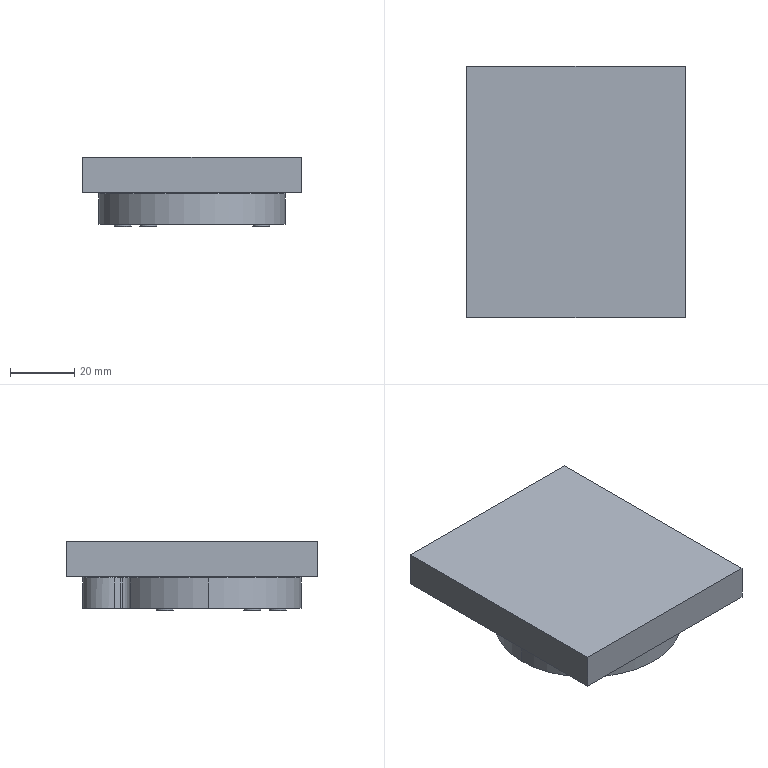NC program | NX | posted with a generic post | part box 68 x 78.27 x 21.8 mm
Lines 1 to 1194 of 3502:
N10 G17 G21 G94 G90
(FLOOR_WALL , TOOL : D80)
N12 T19 M6
N14 G54
N16 G17 G0 G90 X-74. Y0. S5000 M3
N18 G43 Z30. H19
N20 Z3.
N22 G94 G1 Z0. F1200.
N24 X-71.
N26 X71.
N28 X74.
N30 Z3.
N32 G0 Z30.
N34 M5
(CAVITY_MILL , TOOL : D10)
N36 T15 M6
N38 G54
N40 G17 G0 G90 X-37.995 Y9.548 S9500 M3
N42 G43 Z30. H15
N44 Z0.525
N46 G94 G1 Z-0.975 F1000.
N48 X-31.995 Y13.012
N50 G3 X-31.495 Y13.879 R1.
N52 G1 Y36.139 F3500.
N54 G2 X-31.003 Y36.632 R0.492
N56 G1 X31.003
N58 G2 X31.495 Y36.139 R0.492
N60 G1 Y-36.139
N62 G2 X31.003 Y-36.632 R0.492
N64 G1 X-31.003
N66 G2 X-31.495 Y-36.139 R0.492
N68 G1 Y13.879
N70 X-25.495
N72 Y30.632
N74 X25.495
N76 Y-30.632
N78 X-25.495
N80 Y13.879
N82 X-19.495
N84 Y24.632
N86 X19.495
N88 Y-24.632
N90 X9.149
N92 Y-18.632
N94 G3 X13.495 Y-14.286 R16.305
N96 G1 Y-18.632
N98 X9.149
N100 Y-24.632
N102 X-19.495
N104 Y-14.286
N106 X-13.495
N108 G3 X-9.149 Y-18.632 R16.305
N110 G1 X-13.495
N112 Y-14.286
N114 X-19.495
N116 Y13.879
N118 X-13.495
N120 Y18.632
N122 X13.495
N124 Y4.016
N126 G3 X6.155 Y9.964 R16.306
N128 G1 X7.853 Y14.132
N130 X8.995
N132 Y13.626
N134 G3 X7.853 Y14.132 R20.805
N136 G1 X6.155 Y9.964
N138 G3 X-13.495 Y4.016 R16.305
N140 G1 X-12.502 Y3.343
N142 G2 X8.478 Y7.367 R15.105
N144 X-12.502 Y3.343 R-15.105
N146 G1 X-13.495 Y4.016
N148 Y13.879
N150 X-8.995
N152 Y14.132
N154 X-7.853
N156 G3 X-8.995 Y13.626 R20.805
N158 G1 Y13.879
N160 G3 X-9.495 Y14.745 R1.
N162 G1 Z0.525
N164 G0 Z30.
N166 X-37.996 Y9.548
N168 Z-0.45
N170 G1 Z-1.95 F1000.
N172 X-31.996 Y13.013
N174 G3 X-31.496 Y13.879 R1.
N176 G1 Y36.139 F3500.
N178 G2 X-31.003 Y36.632 R0.493
N180 G1 X31.003
N182 G2 X31.496 Y36.139 R0.493
N184 G1 Y-36.139
N186 G2 X31.003 Y-36.632 R0.493
N188 G1 X-31.003
N190 G2 X-31.496 Y-36.139 R0.493
N192 G1 Y13.879
N194 X-25.496
N196 Y30.632
N198 X25.496
N200 Y-30.632
N202 X-25.496
N204 Y13.879
N206 X-19.496
N208 Y24.632
N210 X19.496
N212 Y-24.632
N214 X9.149
N216 Y-18.632
N218 G3 X13.496 Y-14.286 R16.305
N220 G1 Y-18.632
N222 X9.149
N224 Y-24.632
N226 X-19.496
N228 Y-14.286
N230 X-13.496
N232 G3 X-9.149 Y-18.632 R16.305
N234 G1 X-13.496
N236 Y-14.286
N238 X-19.496
N240 Y13.879
N242 X-13.496
N244 Y18.632
N246 X13.496
N248 Y4.016
N250 G3 X6.154 Y9.965 R16.306
N252 G1 X7.853 Y14.132
N254 X8.996
N256 Y13.625
N258 G3 X7.853 Y14.132 R20.805
N260 G1 X6.154 Y9.965
N262 G3 X-13.496 Y4.016 R16.305
N264 G1 X-12.502 Y3.342
N266 G2 X8.477 Y7.368 R15.105
N268 X-12.502 Y3.342 R-15.105
N270 G1 X-13.496 Y4.016
N272 Y13.879
N274 X-8.996
N276 Y14.132
N278 X-7.853
N280 G3 X-8.996 Y13.625 R20.805
N282 G1 Y13.879
N284 G3 X-9.496 Y14.745 R1.
N286 G1 Z-0.45
N288 G0 Z2.025
N290 X-37.996 Y9.548
N292 Z-1.425
N294 G1 Z-2.925 F1000.
N296 X-31.996 Y13.013
N298 G3 X-31.496 Y13.879 R1.
N300 G1 Y36.139 F3500.
N302 G2 X-31.003 Y36.632 R0.493
N304 G1 X31.003
N306 G2 X31.496 Y36.139 R0.493
N308 G1 Y-36.139
N310 G2 X31.003 Y-36.632 R0.493
N312 G1 X-31.003
N314 G2 X-31.496 Y-36.139 R0.493
N316 G1 Y13.879
N318 X-25.496
N320 Y30.632
N322 X25.496
N324 Y-30.632
N326 X-25.496
N328 Y13.879
N330 X-19.496
N332 Y24.632
N334 X19.496
N336 Y-24.632
N338 X9.149
N340 Y-18.632
N342 G3 X13.496 Y-14.285 R16.305
N344 G1 Y-18.632
N346 X9.149
N348 Y-24.632
N350 X-19.496
N352 Y-14.285
N354 X-13.496
N356 G3 X-9.149 Y-18.632 R16.305
N358 G1 X-13.496
N360 Y-14.285
N362 X-19.496
N364 Y13.879
N366 X-13.496
N368 Y18.632
N370 X13.496
N372 Y4.016
N374 G3 X6.154 Y9.965 R16.305
N376 G1 X7.852 Y14.132
N378 X8.996
N380 Y13.625
N382 G3 X7.852 Y14.132 R20.805
N384 G1 X6.154 Y9.965
N386 G3 X-13.496 Y4.016 R16.305
N388 G1 X-12.503 Y3.342
N390 G2 X8.477 Y7.368 R15.105
N392 X-12.503 Y3.342 R-15.105
N394 G1 X-13.496 Y4.016
N396 Y13.879
N398 X-8.996
N400 Y14.132
N402 X-7.852
N404 G3 X-8.996 Y13.625 R20.805
N406 G1 Y13.879
N408 G3 X-9.496 Y14.745 R1.
N410 G1 Z-1.425
N412 G0 Z1.05
N414 X-37.996 Y9.549
N416 Z-2.4
N418 G1 Z-3.9 F1000.
N420 X-31.996 Y13.013
N422 G3 X-31.496 Y13.879 R1.
N424 G1 Y36.139 F3500.
N426 G2 X-31.003 Y36.632 R0.493
N428 G1 X31.003
N430 G2 X31.496 Y36.139 R0.493
N432 G1 Y-36.139
N434 G2 X31.003 Y-36.632 R0.493
N436 G1 X-31.003
N438 G2 X-31.496 Y-36.139 R0.493
N440 G1 Y13.879
N442 X-25.496
N444 Y30.632
N446 X25.496
N448 Y-30.632
N450 X-25.496
N452 Y13.879
N454 X-19.496
N456 Y24.632
N458 X19.496
N460 Y-24.632
N462 X9.148
N464 Y-18.632
N466 G3 X13.496 Y-14.285 R16.305
N468 G1 Y-18.632
N470 X9.148
N472 Y-24.632
N474 X-19.496
N476 Y-14.285
N478 X-13.496
N480 G3 X-9.148 Y-18.632 R16.305
N482 G1 X-13.496
N484 Y-14.285
N486 X-19.496
N488 Y13.879
N490 X-13.496
N492 Y18.632
N494 X13.496
N496 Y4.015
N498 G3 X6.154 Y9.965 R16.305
N500 G1 X7.852 Y14.132
N502 X8.996
N504 Y13.625
N506 G3 X7.852 Y14.132 R20.805
N508 G1 X6.154 Y9.965
N510 G3 X-13.496 Y4.015 R16.305
N512 G1 X-12.503 Y3.342
N514 G2 X8.477 Y7.368 R15.105
N516 X-12.503 Y3.342 R-15.105
N518 G1 X-13.496 Y4.015
N520 Y13.879
N522 X-8.996
N524 Y14.132
N526 X-7.852
N528 G3 X-8.996 Y13.625 R20.805
N530 G1 Y13.879
N532 G3 X-9.496 Y14.745 R1.
N534 G1 Z-2.4
N536 G0 Z0.075
N538 X-4.33 Y43.132
N540 Z-3.4
N542 G1 Z-4.9 F1000.
N544 X-0.866 Y37.132
N546 G3 X0. Y36.632 R1.
N548 G1 X31.003 F3500.
N550 G2 X31.496 Y36.139 R0.494
N552 G1 Y-36.139
N554 G2 X31.003 Y-36.632 R0.494
N556 G1 X-31.003
N558 G2 X-31.496 Y-36.139 R0.494
N560 G1 Y36.139
N562 G2 X-31.003 Y36.632 R0.494
N564 G1 X0.
N566 Y30.632
N568 X25.496
N570 Y-30.632
N572 X-25.496
N574 Y30.632
N576 X0.
N578 Y24.632
N580 X19.496
N582 Y-24.632
N584 X11.604
N586 Y-18.632
N588 G3 X13.496 Y-16.74 R17.8
N590 G1 Y-18.632
N592 X11.604
N594 Y-24.632
N596 X-19.496
N598 Y-16.74
N600 X-13.496
N602 G3 X-11.604 Y-18.632 R17.8
N604 G1 X-13.496
N606 Y-16.74
N608 X-19.496
N610 Y24.632
N612 X0.
N614 Y18.632
N616 X13.496
N618 Y6.471
N620 G3 X-13.496 Y6.471 R17.8
N622 G1 X-12.587 Y5.688
N624 G2 X10.823 Y7.452 R16.6
N626 X-12.587 Y5.688 R-16.6
N628 G1 X-13.496 Y6.471
N630 Y18.632
N632 X0.
N634 G3 X0.866 Y19.132 R1.
N636 G1 Z-3.4
N638 G0 Z-0.9
N640 X-4.33 Y43.133
N642 Z-4.4
N644 G1 Z-5.9 F1000.
N646 X-0.866 Y37.133
N648 G3 X0. Y36.633 R1.
N650 G1 X31.002 F3500.
N652 G2 X31.497 Y36.138 R0.494
N654 G1 Y-36.138
N656 G2 X31.002 Y-36.633 R0.494
N658 G1 X-31.002
N660 G2 X-31.497 Y-36.138 R0.494
N662 G1 Y36.138
N664 G2 X-31.002 Y36.633 R0.494
N666 G1 X0.
N668 Y30.633
N670 X25.497
N672 Y-30.633
N674 X-25.497
N676 Y30.633
N678 X0.
N680 Y24.633
N682 X19.497
N684 Y-24.633
N686 X11.604
N688 Y-18.633
N690 G3 X13.497 Y-16.74 R17.8
N692 G1 Y-18.633
N694 X11.604
N696 Y-24.633
N698 X-19.497
N700 Y-16.74
N702 X-13.497
N704 G3 X-11.604 Y-18.633 R17.8
N706 G1 X-13.497
N708 Y-16.74
N710 X-19.497
N712 Y24.633
N714 X0.
N716 Y18.633
N718 X13.497
N720 Y6.47
N722 G3 X-13.497 Y6.47 R17.8
N724 G1 X-12.587 Y5.688
N726 G2 X10.823 Y7.452 R16.6
N728 X-12.587 Y5.688 R-16.6
N730 G1 X-13.497 Y6.47
N732 Y18.633
N734 X0.
N736 G3 X0.866 Y19.133 R1.
N738 G1 Z-4.4
N740 G0 Z-1.9
N742 X0.317 Y43.133
N744 Z-5.4
N746 G1 Z-6.9 F1000.
N748 X0.133 Y38.465
N750 G3 X0.598 Y37.58 R1.
N752 G1 X2.098 Y36.633 F3500.
N754 X31.002
N756 G2 X31.497 Y36.138 R0.494
N758 G1 Y19.278
N760 X25.497
N762 G3 X7.099 Y29.444 R35.3
N764 X6.744 Y30.633 R14.55
N766 G1 X25.497
N768 Y19.278
N770 X31.497
N772 Y10.804
N774 G2 X31.497 Y-21.073 R35.3
N776 G1 Y-36.138
N778 G2 X31.002 Y-36.633 R0.494
N780 G1 X24.412
N782 Y-30.633
N784 G3 X25.497 Y-29.548 R35.3
N786 G1 Y-30.633
N788 X24.412
N790 Y-36.633
N792 X15.936
N794 G2 X-15.936 Y-36.633 R35.3
N796 G1 X-31.002
N798 G2 X-31.497 Y-36.138 R0.494
N800 G1 Y-29.548
N802 X-25.497
N804 G3 X-24.412 Y-30.633 R35.3
N806 G1 X-25.497
N808 Y-29.548
N810 X-31.497
N812 Y-21.073
N814 G2 X-31.497 Y10.804 R35.3
N816 G1 Y36.138
N818 G2 X-31.002 Y36.633 R0.494
N820 G1 X-20.763
N822 Y30.633
N824 G3 X-21.277 Y23.032 R14.55
N826 X-25.497 Y19.278 R35.3
N828 G1 X-24.63 Y18.448
N830 G2 X-19.938 Y22.529 R34.1
N832 G1 X-20.031 Y22.942
N834 G2 X-5.392 Y39.137 R13.35
N836 X-2.462 Y38.092 R7.1
N838 G1 X2.057 Y35.239
N840 G2 X4.26 Y33.042 R7.1
N842 X6.012 Y28.827 R13.35
N844 G1 X6.106 Y28.414
N846 G2 X-24.63 Y18.448 R-34.1
N848 G1 X-25.497 Y19.278
N850 Y30.633
N852 X-20.763
N854 Y36.633
N856 X-16.817
N858 G2 X-5.247 Y40.328 R14.55
N860 X-1.821 Y39.107 R8.3
N862 G1 X0.598 Y37.58
N864 G3 X1.597 Y37.54 R1.
N866 G1 Y43.133
N868 Z-5.4
N870 G0 Z-2.9
N872 X11.791
N874 Z-6.4
N876 G1 Z-7.9 F1000.
N878 X15.255 Y37.133
N880 G3 X16.121 Y36.633 R1.
N882 G1 X31.002 F3500.
N884 G2 X31.497 Y36.138 R0.495
N886 G1 Y10.803
N888 G2 X31.497 Y-21.073 R35.3
N890 G1 Y-36.138
N892 G2 X31.002 Y-36.633 R0.495
N894 G1 X24.412
N896 Y-30.633
N898 G3 X25.497 Y-29.548 R35.3
N900 G1 Y-30.633
N902 X24.412
N904 Y-36.633
N906 X15.936
N908 G2 X-15.936 Y-36.633 R35.3
N910 G1 X-31.002
N912 G2 X-31.497 Y-36.138 R0.495
N914 G1 Y-29.548
N916 X-25.497
N918 G3 X-24.412 Y-30.633 R35.3
N920 G1 X-25.497
N922 Y-29.548
N924 X-31.497
N926 Y-21.073
N928 G2 X-31.497 Y10.803 R35.3
N930 G1 Y36.138
N932 G2 X-31.002 Y36.633 R0.495
N934 G1 X-20.763
N936 Y30.633
N938 G3 X-21.277 Y23.032 R14.55
N940 X-25.497 Y19.278 R35.3
N942 G1 Y30.633
N944 X-20.763
N946 Y36.633
N948 X-16.816
N950 G2 X-5.247 Y40.328 R14.55
N952 X-1.821 Y39.107 R8.3
N954 G1 X2.097 Y36.633
N956 X16.121
N958 Y30.633
N960 X25.497
N962 Y19.278
N964 G3 X7.099 Y29.444 R35.3
N966 X6.744 Y30.633 R14.55
N968 G1 X5.61 Y30.241
N970 G2 X6.012 Y28.827 R13.35
N972 G1 X6.106 Y28.414
N974 G2 X-19.938 Y22.529 R-34.1
N976 G1 X-20.031 Y22.942
N978 G2 X-5.392 Y39.137 R13.35
N980 X-2.462 Y38.092 R7.1
N982 G1 X2.057 Y35.239
N984 G2 X4.26 Y33.042 R7.1
N986 X5.61 Y30.241 R13.35
N988 G1 X6.744 Y30.633
N990 X16.121
N992 G3 X16.987 Y31.133 R1.
N994 G1 Y43.133
N996 Z-6.4
N998 G0 Z-3.9
N1000 X11.791
N1002 Z-7.4
N1004 G1 Z-8.9 F1000.
N1006 X15.255 Y37.133
N1008 G3 X16.121 Y36.633 R1.
N1010 G1 X31.002 F3500.
N1012 G2 X31.497 Y36.138 R0.495
N1014 G1 Y10.803
N1016 G2 X31.497 Y-21.072 R35.3
N1018 G1 Y-36.138
N1020 G2 X31.002 Y-36.633 R0.495
N1022 G1 X24.412
N1024 Y-30.633
N1026 G3 X25.497 Y-29.547 R35.3
N1028 G1 Y-30.633
N1030 X24.412
N1032 Y-36.633
N1034 X15.936
N1036 G2 X-15.936 Y-36.633 R35.3
N1038 G1 X-31.002
N1040 G2 X-31.497 Y-36.138 R0.495
N1042 G1 Y-29.547
N1044 X-25.497
N1046 G3 X-24.412 Y-30.633 R35.3
N1048 G1 X-25.497
N1050 Y-29.547
N1052 X-31.497
N1054 Y-21.072
N1056 G2 X-31.497 Y10.803 R35.3
N1058 G1 Y36.138
N1060 G2 X-31.002 Y36.633 R0.495
N1062 G1 X-20.763
N1064 Y30.633
N1066 G3 X-21.277 Y23.032 R14.55
N1068 X-25.497 Y19.278 R35.3
N1070 G1 Y30.633
N1072 X-20.763
N1074 Y36.633
N1076 X-16.816
N1078 G2 X-5.247 Y40.328 R14.55
N1080 X-1.821 Y39.107 R8.3
N1082 G1 X2.097 Y36.633
N1084 X16.121
N1086 Y30.633
N1088 X25.497
N1090 Y19.278
N1092 G3 X7.099 Y29.444 R35.3
N1094 X6.744 Y30.633 R14.55
N1096 G1 X5.61 Y30.242
N1098 G2 X6.012 Y28.827 R13.35
N1100 G1 X6.106 Y28.414
N1102 G2 X-19.938 Y22.529 R-34.1
N1104 G1 X-20.031 Y22.942
N1106 G2 X-5.392 Y39.137 R13.35
N1108 X-2.462 Y38.092 R7.1
N1110 G1 X2.057 Y35.239
N1112 G2 X4.26 Y33.042 R7.1
N1114 X5.61 Y30.242 R13.35
N1116 G1 X6.744 Y30.633
N1118 X16.121
N1120 G3 X16.987 Y31.133 R1.
N1122 G1 Y43.133
N1124 Z-7.4
N1126 G0 Z-4.9
N1128 X11.791
N1130 Z-8.4
N1132 G1 Z-9.9 F1000.
N1134 X15.255 Y37.133
N1136 G3 X16.121 Y36.633 R1.
N1138 G1 X31.002 F3500.
N1140 G2 X31.498 Y36.138 R0.496
N1142 G1 Y10.802
N1144 G2 X31.498 Y-21.072 R35.3
N1146 G1 Y-36.138
N1148 G2 X31.002 Y-36.633 R0.496
N1150 G1 X24.411
N1152 Y-30.633
N1154 G3 X25.498 Y-29.547 R35.3
N1156 G1 Y-30.633
N1158 X24.411
N1160 Y-36.633
N1162 X15.935
N1164 G2 X-15.935 Y-36.633 R35.3
N1166 G1 X-31.002
N1168 G2 X-31.498 Y-36.138 R0.496
N1170 G1 Y-29.547
N1172 X-25.498
N1174 G3 X-24.411 Y-30.633 R35.3
N1176 G1 X-25.498
N1178 Y-29.547
N1180 X-31.498
N1182 Y-21.072
N1184 G2 X-31.498 Y10.802 R35.3
N1186 G1 Y36.138
N1188 G2 X-31.002 Y36.633 R0.496
N1190 G1 X-20.763
N1192 Y30.633
N1194 G3 X-21.277 Y23.032 R14.55
N1196 X-25.498 Y19.277 R35.3
N1198 G1 Y30.633
N1200 X-20.763
N1202 Y36.633
N1204 X-16.816
N1206 G2 X-5.247 Y40.328 R14.55
N1208 X-1.821 Y39.107 R8.3
N1210 G1 X2.097 Y36.633
N1212 X16.121
N1214 Y30.633
N1216 X25.498
N1218 Y19.277
N1220 G3 X7.099 Y29.444 R35.3
N1222 X6.744 Y30.633 R14.55
N1224 G1 X5.61 Y30.242
N1226 G2 X6.012 Y28.827 R13.35
N1228 G1 X6.106 Y28.414
N1230 G2 X-19.938 Y22.529 R-34.1
N1232 G1 X-20.031 Y22.942
N1234 G2 X-5.392 Y39.137 R13.35
N1236 X-2.462 Y38.092 R7.1
N1238 G1 X2.057 Y35.239
N1240 G2 X4.26 Y33.042 R7.1
N1242 X5.61 Y30.242 R13.35
N1244 G1 X6.744 Y30.633
N1246 X16.121
N1248 G3 X16.987 Y31.133 R1.
N1250 G1 Y43.133
N1252 Z-8.4
N1254 G0 Z-5.9
N1256 X11.791 Y43.134
N1258 Z-9.4
N1260 G1 Z-10.9 F1000.
N1262 X15.255 Y37.134
N1264 G3 X16.121 Y36.634 R1.
N1266 G1 X31.002 F3500.
N1268 G2 X31.498 Y36.138 R0.496
N1270 G1 Y10.802
N1272 G2 X31.498 Y-21.071 R35.3
N1274 G1 Y-36.138
N1276 G2 X31.002 Y-36.634 R0.496
N1278 G1 X24.411
N1280 Y-30.634
N1282 G3 X25.498 Y-29.547 R35.3
N1284 G1 Y-30.634
N1286 X24.411
N1288 Y-36.634
N1290 X15.935
N1292 G2 X-15.935 Y-36.634 R35.3
N1294 G1 X-31.002
N1296 G2 X-31.498 Y-36.138 R0.496
N1298 G1 Y-29.547
N1300 X-25.498
N1302 G3 X-24.411 Y-30.634 R35.3
N1304 G1 X-25.498
N1306 Y-29.547
N1308 X-31.498
N1310 Y-21.071
N1312 G2 X-31.498 Y10.802 R35.3
N1314 G1 Y36.138
N1316 G2 X-31.002 Y36.634 R0.496
N1318 G1 X-20.763
N1320 Y30.634
N1322 G3 X-21.277 Y23.032 R14.55
N1324 X-25.498 Y19.277 R35.3
N1326 G1 Y30.634
N1328 X-20.763
N1330 Y36.634
N1332 X-16.816
N1334 G2 X-5.247 Y40.328 R14.55
N1336 X-1.821 Y39.107 R8.3
N1338 G1 X2.096 Y36.634
N1340 X16.121
N1342 Y30.634
N1344 X25.498
N1346 Y19.277
N1348 G3 X7.099 Y29.444 R35.3
N1350 X6.744 Y30.634 R14.55
N1352 G1 X5.61 Y30.242
N1354 G2 X6.012 Y28.827 R13.35
N1356 G1 X6.106 Y28.414
N1358 G2 X-19.938 Y22.529 R-34.1
N1360 G1 X-20.031 Y22.942
N1362 G2 X-5.392 Y39.137 R13.35
N1364 X-2.462 Y38.092 R7.1
N1366 G1 X2.057 Y35.239
N1368 G2 X4.26 Y33.042 R7.1
N1370 X5.61 Y30.242 R13.35
N1372 G1 X6.744 Y30.634
N1374 X16.121
N1376 G3 X16.987 Y31.134 R1.
N1378 G1 Y43.134
N1380 Z-9.4
N1382 G0 Z-6.9
N1384 X11.791
N1386 Z-10.4
N1388 G1 Z-11.9 F1000.
N1390 X15.255 Y37.134
N1392 G3 X16.121 Y36.634 R1.
N1394 G1 X31.002 F3500.
N1396 G2 X31.498 Y36.138 R0.496
N1398 G1 Y10.801
N1400 G2 X31.498 Y-21.071 R35.3
N1402 G1 Y-36.138
N1404 G2 X31.002 Y-36.634 R0.496
N1406 G1 X24.411
N1408 Y-30.634
N1410 G3 X25.498 Y-29.547 R35.3
N1412 G1 Y-30.634
N1414 X24.411
N1416 Y-36.634
N1418 X15.934
N1420 G2 X-15.934 Y-36.634 R35.3
N1422 G1 X-31.002
N1424 G2 X-31.498 Y-36.138 R0.496
N1426 G1 Y-29.547
N1428 X-25.498
N1430 G3 X-24.411 Y-30.634 R35.3
N1432 G1 X-25.498
N1434 Y-29.547
N1436 X-31.498
N1438 Y-21.071
N1440 G2 X-31.498 Y10.801 R35.3
N1442 G1 Y36.138
N1444 G2 X-31.002 Y36.634 R0.496
N1446 G1 X-20.762
N1448 Y30.634
N1450 G3 X-21.277 Y23.032 R14.55
N1452 X-25.498 Y19.277 R35.3
N1454 G1 Y30.634
N1456 X-20.762
N1458 Y36.634
N1460 X-16.815
N1462 G2 X-5.247 Y40.328 R14.55
N1464 X-1.821 Y39.107 R8.3
N1466 G1 X2.096 Y36.634
N1468 X16.121
N1470 Y30.634
N1472 X25.498
N1474 Y19.277
N1476 G3 X7.099 Y29.444 R35.3
N1478 X6.744 Y30.634 R14.55
N1480 G1 X5.61 Y30.242
N1482 G2 X6.012 Y28.827 R13.35
N1484 G1 X6.106 Y28.414
N1486 G2 X-19.938 Y22.529 R-34.1
N1488 G1 X-20.031 Y22.942
N1490 G2 X-5.392 Y39.137 R13.35
N1492 X-2.462 Y38.092 R7.1
N1494 G1 X2.057 Y35.239
N1496 G2 X4.26 Y33.042 R7.1
N1498 X5.61 Y30.242 R13.35
N1500 G1 X6.744 Y30.634
N1502 X16.121
N1504 G3 X16.987 Y31.134 R1.
N1506 G1 Y43.134
N1508 Z-10.4
N1510 G0 Z-7.9
N1512 X11.791
N1514 Z-11.4
N1516 G1 Z-12.9 F1000.
N1518 X15.255 Y37.134
N1520 G3 X16.121 Y36.634 R1.
N1522 G1 X31.002 F3500.
N1524 G2 X31.498 Y36.137 R0.497
N1526 G1 Y10.801
N1528 G2 X31.498 Y-21.071 R35.3
N1530 G1 Y-36.137
N1532 G2 X31.002 Y-36.634 R0.497
N1534 G1 X24.411
N1536 Y-30.634
N1538 G3 X25.498 Y-29.546 R35.3
N1540 G1 Y-30.634
N1542 X24.411
N1544 Y-36.634
N1546 X15.934
N1548 G2 X-15.934 Y-36.634 R35.3
N1550 G1 X-31.002
N1552 G2 X-31.498 Y-36.137 R0.497
N1554 G1 Y-29.546
N1556 X-25.498
N1558 G3 X-24.411 Y-30.634 R35.3
N1560 G1 X-25.498
N1562 Y-29.546
N1564 X-31.498
N1566 Y-21.071
N1568 G2 X-31.498 Y10.801 R35.3
N1570 G1 Y36.137
N1572 G2 X-31.002 Y36.634 R0.497
N1574 G1 X-20.762
N1576 Y30.634
N1578 G3 X-21.277 Y23.032 R14.55
N1580 X-25.498 Y19.277 R35.3
N1582 G1 Y30.634
N1584 X-20.762
N1586 Y36.634
N1588 X-16.815
N1590 G2 X-5.247 Y40.328 R14.55
N1592 X-1.821 Y39.107 R8.3
N1594 G1 X2.096 Y36.634
N1596 X16.121
N1598 Y30.634
N1600 X25.498
N1602 Y19.277
N1604 G3 X7.099 Y29.444 R35.3
N1606 X6.744 Y30.634 R14.55
N1608 G1 X5.61 Y30.242
N1610 G2 X6.012 Y28.827 R13.35
N1612 G1 X6.106 Y28.414
N1614 G2 X-19.938 Y22.529 R-34.1
N1616 G1 X-20.031 Y22.942
N1618 G2 X-5.392 Y39.137 R13.35
N1620 X-2.462 Y38.092 R7.1
N1622 G1 X2.057 Y35.239
N1624 G2 X4.26 Y33.042 R7.1
N1626 X5.61 Y30.242 R13.35
N1628 G1 X6.744 Y30.634
N1630 X16.121
N1632 G3 X16.987 Y31.134 R1.
N1634 G1 Y43.134
N1636 Z-11.4
N1638 G0 Z-8.9
N1640 X11.791
N1642 Z-12.375
N1644 G1 Z-13.875 F1000.
N1646 X15.255 Y37.134
N1648 G3 X16.121 Y36.634 R1.
N1650 G1 X31.002 F3500.
N1652 G2 X31.499 Y36.137 R0.497
N1654 G1 Y10.8
N1656 G2 X31.499 Y-21.07 R35.3
N1658 G1 Y-36.137
N1660 G2 X31.002 Y-36.634 R0.497
N1662 G1 X24.41
N1664 Y-30.634
N1666 G3 X25.499 Y-29.546 R35.3
N1668 G1 Y-30.634
N1670 X24.41
N1672 Y-36.634
N1674 X15.934
N1676 G2 X-15.934 Y-36.634 R35.3
N1678 G1 X-31.002
N1680 G2 X-31.499 Y-36.137 R0.497
N1682 G1 Y-29.546
N1684 X-25.499
N1686 G3 X-24.41 Y-30.634 R35.3
N1688 G1 X-25.499
N1690 Y-29.546
N1692 X-31.499
N1694 Y-21.07
N1696 G2 X-31.499 Y10.8 R35.3
N1698 G1 Y36.137
N1700 G2 X-31.002 Y36.634 R0.497
N1702 G1 X-20.762
N1704 Y30.634
N1706 G3 X-21.277 Y23.032 R14.55
N1708 X-25.499 Y19.276 R35.3
N1710 G1 Y30.634
N1712 X-20.762
N1714 Y36.634
N1716 X-16.815
N1718 G2 X-5.247 Y40.328 R14.55
N1720 X-1.821 Y39.107 R8.3
N1722 G1 X2.095 Y36.634
N1724 X16.121
N1726 Y30.634
N1728 X25.499
N1730 Y19.276
N1732 G3 X7.099 Y29.444 R35.3
N1734 X6.744 Y30.634 R14.55
N1736 G1 X5.61 Y30.243
N1738 G2 X6.012 Y28.827 R13.35
N1740 G1 X6.106 Y28.414
N1742 G2 X-19.938 Y22.529 R-34.1
N1744 G1 X-20.031 Y22.942
N1746 G2 X-5.392 Y39.137 R13.35
N1748 X-2.462 Y38.092 R7.1
N1750 G1 X2.057 Y35.239
N1752 G2 X4.26 Y33.042 R7.1
N1754 X5.61 Y30.243 R13.35
N1756 G1 X6.744 Y30.634
N1758 X16.121
N1760 G3 X16.987 Y31.134 R1.
N1762 G1 Y43.134
N1764 Z-12.375
N1766 G0 Z-9.9
N1768 X11.791
N1770 Z-13.35
N1772 G1 Z-14.85 F1000.
N1774 X15.255 Y37.134
N1776 G3 X16.121 Y36.634 R1.
N1778 G1 X31.001 F3500.
N1780 G2 X31.499 Y36.137 R0.497
N1782 G1 Y10.8
N1784 G2 X31.499 Y-21.07 R35.3
N1786 G1 Y-36.137
N1788 G2 X31.001 Y-36.634 R0.497
N1790 G1 X24.41
N1792 Y-30.634
N1794 G3 X25.499 Y-29.546 R35.3
N1796 G1 Y-30.634
N1798 X24.41
N1800 Y-36.634
N1802 X15.933
N1804 G2 X-15.933 Y-36.634 R35.3
N1806 G1 X-31.001
N1808 G2 X-31.499 Y-36.137 R0.497
N1810 G1 Y-29.546
N1812 X-25.499
N1814 G3 X-24.41 Y-30.634 R35.3
N1816 G1 X-25.499
N1818 Y-29.546
N1820 X-31.499
N1822 Y-21.07
N1824 G2 X-31.499 Y10.8 R35.3
N1826 G1 Y36.137
N1828 G2 X-31.001 Y36.634 R0.497
N1830 G1 X-20.762
N1832 Y30.634
N1834 G3 X-21.277 Y23.032 R14.55
N1836 X-25.499 Y19.276 R35.3
N1838 G1 Y30.634
N1840 X-20.762
N1842 Y36.634
N1844 X-16.815
N1846 G2 X-5.247 Y40.328 R14.55
N1848 X-1.821 Y39.107 R8.3
N1850 G1 X2.095 Y36.634
N1852 X16.121
N1854 Y30.634
N1856 X25.499
N1858 Y19.276
N1860 G3 X7.099 Y29.444 R35.3
N1862 X6.744 Y30.634 R14.55
N1864 G1 X5.609 Y30.243
N1866 G2 X6.012 Y28.827 R13.35
N1868 G1 X6.106 Y28.414
N1870 G2 X-19.938 Y22.529 R-34.1
N1872 G1 X-20.031 Y22.942
N1874 G2 X-5.392 Y39.137 R13.35
N1876 X-2.462 Y38.092 R7.1
N1878 G1 X2.057 Y35.239
N1880 G2 X4.26 Y33.042 R7.1
N1882 X5.609 Y30.243 R13.35
N1884 G1 X6.744 Y30.634
N1886 X16.121
N1888 G3 X16.987 Y31.134 R1.
N1890 G1 Y43.134
N1892 Z-13.35
N1894 G0 Z-10.875
N1896 X11.791 Y43.135
N1898 Z-14.325
N1900 G1 Z-15.825 F1000.
N1902 X15.255 Y37.135
N1904 G3 X16.121 Y36.635 R1.
N1906 G1 X31.001 F3500.
N1908 G2 X31.499 Y36.137 R0.498
N1910 G1 Y10.799
N1912 G2 X31.499 Y-21.069 R35.3
N1914 G1 Y-36.137
N1916 G2 X31.001 Y-36.635 R0.498
N1918 G1 X24.41
N1920 Y-30.635
N1922 G3 X25.499 Y-29.546 R35.3
N1924 G1 Y-30.635
N1926 X24.41
N1928 Y-36.635
N1930 X15.933
N1932 G2 X-15.933 Y-36.635 R35.3
N1934 G1 X-31.001
N1936 G2 X-31.499 Y-36.137 R0.498
N1938 G1 Y-29.546
N1940 X-25.499
N1942 G3 X-24.41 Y-30.635 R35.3
N1944 G1 X-25.499
N1946 Y-29.546
N1948 X-31.499
N1950 Y-21.069
N1952 G2 X-31.499 Y10.799 R35.3
N1954 G1 Y36.137
N1956 G2 X-31.001 Y36.635 R0.498
N1958 G1 X-20.762
N1960 Y30.635
N1962 G3 X-21.277 Y23.032 R14.55
N1964 X-25.499 Y19.276 R35.3
N1966 G1 Y30.635
N1968 X-20.762
N1970 Y36.635
N1972 X-16.815
N1974 G2 X-5.247 Y40.328 R14.55
N1976 X-1.821 Y39.107 R8.3
N1978 G1 X2.095 Y36.635
N1980 X16.121
N1982 Y30.635
N1984 X25.499
N1986 Y19.276
N1988 G3 X7.099 Y29.444 R35.3
N1990 X6.744 Y30.635 R14.55
N1992 G1 X5.609 Y30.243
N1994 G2 X6.012 Y28.827 R13.35
N1996 G1 X6.106 Y28.414
N1998 G2 X-19.938 Y22.529 R-34.1
N2000 G1 X-20.031 Y22.942
N2002 G2 X-5.392 Y39.137 R13.35
N2004 X-2.462 Y38.092 R7.1
N2006 G1 X2.057 Y35.239
N2008 G2 X4.26 Y33.042 R7.1
N2010 X5.609 Y30.243 R13.35
N2012 G1 X6.744 Y30.635
N2014 X16.121
N2016 G3 X16.987 Y31.135 R1.
N2018 G1 Y43.135
N2020 Z-14.325
N2022 G0 Z-11.85
N2024 X11.791
N2026 Z-15.3
N2028 G1 Z-16.8 F1000.
N2030 X15.255 Y37.135
N2032 G3 X16.121 Y36.635 R1.
N2034 G1 X31.001 F3500.
N2036 G2 X31.499 Y36.137 R0.498
N2038 G1 Y10.799
N2040 G2 X31.499 Y-21.069 R35.3
N2042 G1 Y-36.137
N2044 G2 X31.001 Y-36.635 R0.498
N2046 G1 X24.41
N2048 Y-30.635
N2050 G3 X25.499 Y-29.545 R35.3
N2052 G1 Y-30.635
N2054 X24.41
N2056 Y-36.635
N2058 X15.932
N2060 G2 X-15.932 Y-36.635 R35.3
N2062 G1 X-31.001
N2064 G2 X-31.499 Y-36.137 R0.498
N2066 G1 Y-29.545
N2068 X-25.499
N2070 G3 X-24.41 Y-30.635 R35.3
N2072 G1 X-25.499
N2074 Y-29.545
N2076 X-31.499
N2078 Y-21.069
N2080 G2 X-31.499 Y10.799 R35.3
N2082 G1 Y36.137
N2084 G2 X-31.001 Y36.635 R0.498
N2086 G1 X-20.762
N2088 Y30.635
N2090 G3 X-21.277 Y23.032 R14.55
N2092 X-25.499 Y19.276 R35.3
N2094 G1 Y30.635
N2096 X-20.762
N2098 Y36.635
N2100 X-16.814
N2102 G2 X-5.247 Y40.328 R14.55
N2104 X-1.821 Y39.107 R8.3
N2106 G1 X2.094 Y36.635
N2108 X16.121
N2110 Y30.635
N2112 X25.499
N2114 Y19.276
N2116 G3 X7.099 Y29.444 R35.3
N2118 X6.744 Y30.635 R14.55
N2120 G1 X5.609 Y30.243
N2122 G2 X6.012 Y28.827 R13.35
N2124 G1 X6.106 Y28.414
N2126 G2 X-19.938 Y22.529 R-34.1
N2128 G1 X-20.031 Y22.942
N2130 G2 X-5.392 Y39.137 R13.35
N2132 X-2.462 Y38.092 R7.1
N2134 G1 X2.057 Y35.239
N2136 G2 X4.26 Y33.042 R7.1
N2138 X5.609 Y30.243 R13.35
N2140 G1 X6.744 Y30.635
N2142 X16.121
N2144 G3 X16.987 Y31.135 R1.
N2146 G1 Y43.135
N2148 Z-15.3
N2150 G0 Z30.
(FLOOR_WALL_1 , TOOL : D10)
N2152 X0. Y-24.635
N2154 Z-1.
N2156 G1 Z-4. F1000.
N2158 Y-20.64
N2160 G2 X-15.506 Y-5.135 R15.506 F1250.
N2162 X0. Y-20.64 R-15.506
N2164 G1 Y-24.635
N2166 Y-20.14 F1000.
N2168 G2 X-15.006 Y-5.135 R15.006 F1250.
N2170 X0. Y-20.14 R-15.006
N2172 G1 Y-23.64
N2174 Z-1.
N2176 G0 Z30.
N2178 X-19.486 Y-35.998
N2180 Z-3.
N2182 G1 Z-6. F1000.
N2184 X-17.885 Y-33.461
N2186 X-22.112 Y-30.792 F1250.
N2188 X-21.912 Y-30.475
N2190 G2 X-30.679 Y8.322 R33.5
N2192 G1 X-30.996 Y8.522
N2194 X-25.657 Y16.978
N2196 X-25.34 Y16.777
N2198 G2 X-19.264 Y22.272 R33.5
N2200 G1 X-19.446 Y23.075
N2202 G2 X-5.465 Y38.541 R12.75
N2204 X-2.782 Y37.585 R6.5
N2206 G1 X1.737 Y34.732
N2208 G2 X3.753 Y32.721 R6.5
N2210 X5.427 Y28.695 R12.75
N2212 G1 X5.609 Y27.892
N2214 G2 X30.679 Y-18.591 R33.5
N2216 G1 X30.996 Y-18.792
N2218 X25.657 Y-27.247
N2220 X25.34 Y-27.047
N2222 G2 X-13.456 Y-35.813 R33.5
N2224 G1 X-13.657 Y-36.131
N2226 X-17.885 Y-33.461
N2228 X-15.215 Y-29.234
N2230 X-17.836 Y-27.579
N2232 G3 X-18.642 Y-26.693 R5.
N2234 G2 X-26.1 Y6.313 R28.5
N2236 G3 X-25.753 Y7.459 R5.
N2238 G1 X-22.444 Y12.701
N2240 G3 X-21.558 Y13.507 R5.
N2242 G2 X-16.389 Y18.181 R28.5
N2244 G3 X-14.387 Y23.374 R5.
N2246 G1 X-14.569 Y24.177
N2248 G2 X-6.071 Y33.578 R7.75
N2250 X-5.452 Y33.357 R1.5
N2252 G1 X-0.933 Y30.504
N2254 G2 X-0.467 Y30.04 R1.5
N2256 X0.55 Y27.593 R7.75
N2258 G1 X0.732 Y26.79
N2260 G3 X4.771 Y22.963 R5.
N2262 G2 X26.1 Y-16.583 R28.5
N2264 G3 X25.753 Y-17.729 R5.
N2266 G1 X22.444 Y-22.971
N2268 G3 X21.558 Y-23.776 R5.
N2270 G2 X-11.448 Y-31.235 R28.5
N2272 G3 X-12.594 Y-30.888 R5.
N2274 G1 X-15.215 Y-29.234
N2276 X-12.546 Y-25.006
N2278 X-14.479 Y-23.785
N2280 G3 X-15.371 Y-22.911 R10.
N2282 G2 X-21.521 Y4.305 R23.5
N2284 G3 X-21.091 Y5.478 R10.
N2286 G1 X-18.65 Y9.344
N2288 G3 X-17.776 Y10.236 R10.
N2290 G2 X-13.514 Y14.091 R23.5
N2292 G3 X-9.51 Y24.476 R10.
N2294 G1 X-9.692 Y25.279
N2296 G2 X-7.311 Y28.618 R2.75
N2298 G1 X-4.412 Y26.787
N2300 G2 X-4.327 Y26.491 R2.75
N2302 G1 X-4.146 Y25.688
N2304 G3 X3.934 Y18.033 R10.
N2306 G2 X21.521 Y-14.574 R23.5
N2308 G3 X21.091 Y-15.747 R10.
N2310 G1 X18.65 Y-19.614
N2312 G3 X17.776 Y-20.506 R10.
N2314 G2 X-9.44 Y-26.656 R23.5
N2316 G3 X-10.613 Y-26.226 R10.
N2318 G1 X-12.546 Y-25.006
N2320 X-9.877 Y-20.778
N2322 X-11.285 Y-19.888
N2324 G3 X-12.101 Y-19.129 R15.
N2326 G2 X-16.942 Y2.296 R18.5
N2328 G3 X-16.532 Y3.333 R15.
N2330 G1 X-14.754 Y6.15
N2332 G3 X-13.994 Y6.965 R15.
N2334 G2 X-10.639 Y10. R18.5
N2336 G3 X-5.086 Y17.375 R15.
N2338 X3.097 Y13.104 R15.
N2340 G2 X16.942 Y-12.566 R18.5
N2342 G3 X16.532 Y-13.603 R15.
N2344 G1 X14.754 Y-16.42
N2346 G3 X13.994 Y-17.236 R15.
N2348 G2 X-7.431 Y-22.077 R18.5
N2350 G3 X-8.468 Y-21.667 R15.
N2352 G1 X-9.877 Y-20.778
N2354 X-9.076 Y-19.51
N2356 G2 X-14.375 Y3.941 R17.
N2358 X-9.076 Y-19.51 R-17.
N2360 G1 X-10.677 Y-22.046
N2362 X-8.809 Y-19.087 F1000.
N2364 G2 X-13.952 Y3.674 R16.5 F1250.
N2366 X-8.809 Y-19.087 R-16.5
N2368 G1 X-10.677 Y-22.046
N2370 Z-3.
N2372 G0 Z30.
N2374 M5